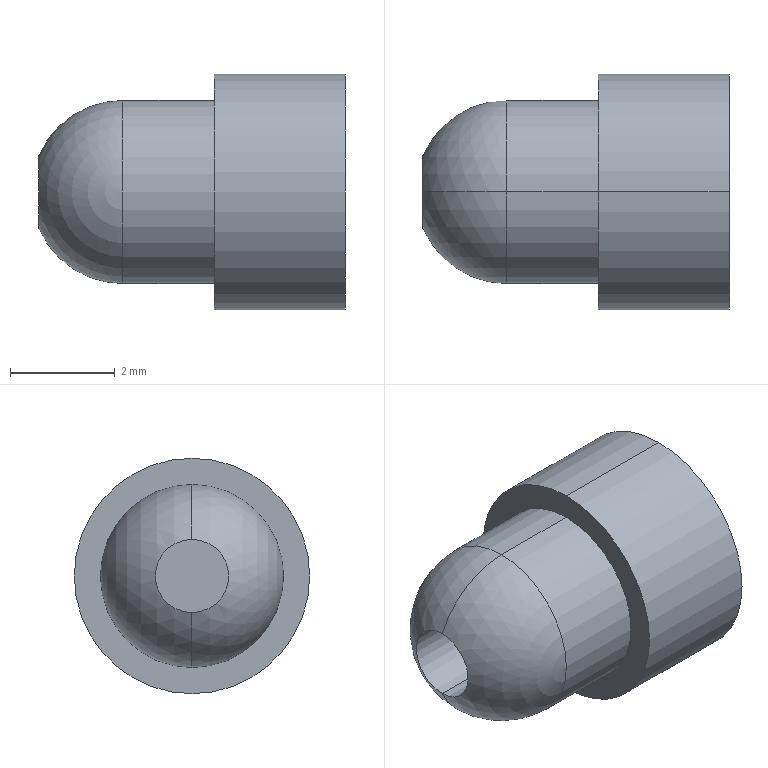Part | NX | 1 solid | 11 faces | box 5.854 x 4.5 x 4.5 mm | volume 60.236 mm3 | cylinder 6 | plane 3 | sphere 2 | commonest cylinder face diameters 1.4 x2 3.5 x2 4.5 x2
STEP:
#1=CARTESIAN_POINT('',(-7.75,0.,23.75));
#2=VERTEX_POINT('',#1);
#3=CARTESIAN_POINT('',(-7.75,0.,28.25));
#4=VERTEX_POINT('',#3);
#5=CARTESIAN_POINT('',(-7.75,0.,26.));
#6=DIRECTION('',(1.,0.,0.));
#7=DIRECTION('',(0.,0.,1.));
#8=AXIS2_PLACEMENT_3D('',#5,#6,#7);
#9=CIRCLE('',#8,2.25);
#10=EDGE_CURVE('',#2,#4,#9,.T.);
#11=ORIENTED_EDGE('',*,*,#10,.T.);
#12=CARTESIAN_POINT('',(-7.75,0.,26.));
#13=DIRECTION('',(1.,0.,0.));
#14=DIRECTION('',(0.,0.,1.));
#15=AXIS2_PLACEMENT_3D('',#12,#13,#14);
#16=CIRCLE('',#15,2.25);
#17=EDGE_CURVE('',#4,#2,#16,.T.);
#18=ORIENTED_EDGE('',*,*,#17,.T.);
#19=EDGE_LOOP('',(#11,#18));
#20=FACE_BOUND('',#19,.T.);
#21=CARTESIAN_POINT('',(-7.75,0.,26.));
#22=DIRECTION('',(1.,0.,0.));
#23=DIRECTION('',(0.,1.,0.));
#24=AXIS2_PLACEMENT_3D('',#21,#22,#23);
#25=PLANE('',#24);
#26=ADVANCED_FACE('',(#20),#25,.T.);
#27=CARTESIAN_POINT('',(-8.75,0.,25.3));
#28=VERTEX_POINT('',#27);
#29=CARTESIAN_POINT('',(-8.75,0.,26.7));
#30=VERTEX_POINT('',#29);
#31=CARTESIAN_POINT('',(-8.75,0.,26.));
#32=DIRECTION('',(-1.,0.,0.));
#33=DIRECTION('',(0.,0.,1.));
#34=AXIS2_PLACEMENT_3D('',#31,#32,#33);
#35=CIRCLE('',#34,0.7);
#36=EDGE_CURVE('',#28,#30,#35,.T.);
#37=ORIENTED_EDGE('',*,*,#36,.T.);
#38=CARTESIAN_POINT('',(-8.75,0.,26.));
#39=DIRECTION('',(-1.,0.,0.));
#40=DIRECTION('',(0.,0.,1.));
#41=AXIS2_PLACEMENT_3D('',#38,#39,#40);
#42=CIRCLE('',#41,0.7);
#43=EDGE_CURVE('',#30,#28,#42,.T.);
#44=ORIENTED_EDGE('',*,*,#43,.T.);
#45=EDGE_LOOP('',(#37,#44));
#46=FACE_BOUND('',#45,.T.);
#47=CARTESIAN_POINT('',(-8.75,0.,26.));
#48=DIRECTION('',(-1.,0.,0.));
#49=DIRECTION('',(0.,0.,1.));
#50=AXIS2_PLACEMENT_3D('',#47,#48,#49);
#51=PLANE('',#50);
#52=ADVANCED_FACE('',(#46),#51,.T.);
#53=CARTESIAN_POINT('',(-10.25,0.,28.25));
#54=VERTEX_POINT('',#53);
#55=CARTESIAN_POINT('',(-10.25,0.,23.75));
#56=VERTEX_POINT('',#55);
#57=CARTESIAN_POINT('',(-10.25,0.,26.));
#58=DIRECTION('',(-1.,0.,0.));
#59=DIRECTION('',(0.,0.,1.));
#60=AXIS2_PLACEMENT_3D('',#57,#58,#59);
#61=CIRCLE('',#60,2.25);
#62=EDGE_CURVE('',#54,#56,#61,.T.);
#63=ORIENTED_EDGE('',*,*,#62,.F.);
#64=CARTESIAN_POINT('',(-9.5,0.,28.25));
#65=DIRECTION('',(-1.,0.,0.));
#66=VECTOR('',#65,1000.);
#67=LINE('',#64,#66);
#68=EDGE_CURVE('',#4,#54,#67,.T.);
#69=ORIENTED_EDGE('',*,*,#68,.F.);
#70=ORIENTED_EDGE('',*,*,#10,.F.);
#71=CARTESIAN_POINT('',(-9.5,0.,23.75));
#72=DIRECTION('',(-1.,0.,0.));
#73=VECTOR('',#72,1000.);
#74=LINE('',#71,#73);
#75=EDGE_CURVE('',#2,#56,#74,.T.);
#76=ORIENTED_EDGE('',*,*,#75,.T.);
#77=EDGE_LOOP('',(#63,#69,#70,#76));
#78=FACE_BOUND('',#77,.T.);
#79=CARTESIAN_POINT('',(-9.5,0.,26.));
#80=DIRECTION('',(-1.,0.,0.));
#81=DIRECTION('',(0.,0.,1.));
#82=AXIS2_PLACEMENT_3D('',#79,#80,#81);
#83=CYLINDRICAL_SURFACE('',#82,2.25);
#84=ADVANCED_FACE('',(#78),#83,.T.);
#85=CARTESIAN_POINT('',(-12.,0.,24.25));
#86=VERTEX_POINT('',#85);
#87=CARTESIAN_POINT('',(-12.,0.,27.75));
#88=VERTEX_POINT('',#87);
#89=CARTESIAN_POINT('',(-12.,0.,26.));
#90=DIRECTION('',(-1.,0.,0.));
#91=DIRECTION('',(0.,0.,1.));
#92=AXIS2_PLACEMENT_3D('',#89,#90,#91);
#93=CIRCLE('',#92,1.75);
#94=EDGE_CURVE('',#86,#88,#93,.T.);
#95=ORIENTED_EDGE('',*,*,#94,.F.);
#96=CARTESIAN_POINT('',(-10.25,0.,24.25));
#97=VERTEX_POINT('',#96);
#98=CARTESIAN_POINT('',(-11.125,0.,24.25));
#99=DIRECTION('',(-1.,0.,0.));
#100=VECTOR('',#99,1000.);
#101=LINE('',#98,#100);
#102=EDGE_CURVE('',#97,#86,#101,.T.);
#103=ORIENTED_EDGE('',*,*,#102,.F.);
#104=CARTESIAN_POINT('',(-10.25,0.,27.75));
#105=VERTEX_POINT('',#104);
#106=CARTESIAN_POINT('',(-10.25,0.,26.));
#107=DIRECTION('',(-1.,0.,0.));
#108=DIRECTION('',(0.,0.,1.));
#109=AXIS2_PLACEMENT_3D('',#106,#107,#108);
#110=CIRCLE('',#109,1.75);
#111=EDGE_CURVE('',#97,#105,#110,.T.);
#112=ORIENTED_EDGE('',*,*,#111,.T.);
#113=CARTESIAN_POINT('',(-11.125,0.,27.75));
#114=DIRECTION('',(-1.,0.,0.));
#115=VECTOR('',#114,1000.);
#116=LINE('',#113,#115);
#117=EDGE_CURVE('',#105,#88,#116,.T.);
#118=ORIENTED_EDGE('',*,*,#117,.T.);
#119=EDGE_LOOP('',(#95,#103,#112,#118));
#120=FACE_BOUND('',#119,.T.);
#121=CARTESIAN_POINT('',(-11.125,0.,26.));
#122=DIRECTION('',(-1.,0.,0.));
#123=DIRECTION('',(0.,0.,1.));
#124=AXIS2_PLACEMENT_3D('',#121,#122,#123);
#125=CYLINDRICAL_SURFACE('',#124,1.75);
#126=ADVANCED_FACE('',(#120),#125,.T.);
#127=ORIENTED_EDGE('',*,*,#36,.F.);
#128=CARTESIAN_POINT('',(-13.604,0.,25.3));
#129=VERTEX_POINT('',#128);
#130=CARTESIAN_POINT('',(-11.25,0.,25.3));
#131=DIRECTION('',(-1.,0.,0.));
#132=VECTOR('',#131,1000.);
#133=LINE('',#130,#132);
#134=EDGE_CURVE('',#129,#28,#133,.F.);
#135=ORIENTED_EDGE('',*,*,#134,.F.);
#136=CARTESIAN_POINT('',(-13.604,0.,26.7));
#137=VERTEX_POINT('',#136);
#138=CARTESIAN_POINT('',(-13.604,0.,26.));
#139=DIRECTION('',(1.,0.,0.));
#140=DIRECTION('',(0.,0.,1.));
#141=AXIS2_PLACEMENT_3D('',#138,#139,#140);
#142=CIRCLE('',#141,0.7);
#143=EDGE_CURVE('',#137,#129,#142,.T.);
#144=ORIENTED_EDGE('',*,*,#143,.F.);
#145=CARTESIAN_POINT('',(-11.25,0.,26.7));
#146=DIRECTION('',(-1.,0.,0.));
#147=VECTOR('',#146,1000.);
#148=LINE('',#145,#147);
#149=EDGE_CURVE('',#137,#30,#148,.F.);
#150=ORIENTED_EDGE('',*,*,#149,.T.);
#151=EDGE_LOOP('',(#127,#135,#144,#150));
#152=FACE_BOUND('',#151,.T.);
#153=CARTESIAN_POINT('',(-11.25,0.,26.));
#154=DIRECTION('',(-1.,0.,0.));
#155=DIRECTION('',(0.,0.,1.));
#156=AXIS2_PLACEMENT_3D('',#153,#154,#155);
#157=CYLINDRICAL_SURFACE('',#156,0.7);
#158=ADVANCED_FACE('',(#152),#157,.F.);
#159=CARTESIAN_POINT('',(-12.,0.,26.));
#160=DIRECTION('',(-1.,0.,0.));
#161=DIRECTION('',(0.,0.,1.));
#162=AXIS2_PLACEMENT_3D('',#159,#160,#161);
#163=CIRCLE('',#162,1.75);
#164=EDGE_CURVE('',#88,#86,#163,.T.);
#165=ORIENTED_EDGE('',*,*,#164,.T.);
#166=CARTESIAN_POINT('',(-12.,0.,26.));
#167=DIRECTION('',(0.,1.,0.));
#168=DIRECTION('',(1.,0.,0.));
#169=AXIS2_PLACEMENT_3D('',#166,#167,#168);
#170=CIRCLE('',#169,1.75);
#171=EDGE_CURVE('',#86,#129,#170,.T.);
#172=ORIENTED_EDGE('',*,*,#171,.T.);
#173=CARTESIAN_POINT('',(-13.604,0.,26.));
#174=DIRECTION('',(1.,0.,0.));
#175=DIRECTION('',(0.,0.,1.));
#176=AXIS2_PLACEMENT_3D('',#173,#174,#175);
#177=CIRCLE('',#176,0.7);
#178=EDGE_CURVE('',#129,#137,#177,.T.);
#179=ORIENTED_EDGE('',*,*,#178,.T.);
#180=CARTESIAN_POINT('',(-12.,0.,26.));
#181=DIRECTION('',(0.,1.,0.));
#182=DIRECTION('',(1.,0.,0.));
#183=AXIS2_PLACEMENT_3D('',#180,#181,#182);
#184=CIRCLE('',#183,1.75);
#185=EDGE_CURVE('',#137,#88,#184,.T.);
#186=ORIENTED_EDGE('',*,*,#185,.T.);
#187=EDGE_LOOP('',(#165,#172,#179,#186));
#188=FACE_BOUND('',#187,.T.);
#189=CARTESIAN_POINT('',(-12.,0.,26.));
#190=DIRECTION('',(0.,1.,0.));
#191=DIRECTION('',(1.,0.,0.));
#192=AXIS2_PLACEMENT_3D('',#189,#190,#191);
#193=SPHERICAL_SURFACE('',#192,1.75);
#194=ADVANCED_FACE('',(#188),#193,.T.);
#195=ORIENTED_EDGE('',*,*,#62,.T.);
#196=CARTESIAN_POINT('',(-10.25,0.,26.));
#197=DIRECTION('',(-1.,0.,0.));
#198=DIRECTION('',(0.,0.,1.));
#199=AXIS2_PLACEMENT_3D('',#196,#197,#198);
#200=CIRCLE('',#199,2.25);
#201=EDGE_CURVE('',#56,#54,#200,.T.);
#202=ORIENTED_EDGE('',*,*,#201,.T.);
#203=EDGE_LOOP('',(#195,#202));
#204=FACE_BOUND('',#203,.T.);
#205=ORIENTED_EDGE('',*,*,#111,.F.);
#206=CARTESIAN_POINT('',(-10.25,0.,26.));
#207=DIRECTION('',(-1.,0.,0.));
#208=DIRECTION('',(0.,0.,1.));
#209=AXIS2_PLACEMENT_3D('',#206,#207,#208);
#210=CIRCLE('',#209,1.75);
#211=EDGE_CURVE('',#105,#97,#210,.T.);
#212=ORIENTED_EDGE('',*,*,#211,.F.);
#213=EDGE_LOOP('',(#205,#212));
#214=FACE_BOUND('',#213,.T.);
#215=CARTESIAN_POINT('',(-10.25,0.,28.));
#216=DIRECTION('',(-1.,0.,0.));
#217=DIRECTION('',(0.,0.,1.));
#218=AXIS2_PLACEMENT_3D('',#215,#216,#217);
#219=PLANE('',#218);
#220=ADVANCED_FACE('',(#204,#214),#219,.T.);
#221=ORIENTED_EDGE('',*,*,#68,.T.);
#222=ORIENTED_EDGE('',*,*,#201,.F.);
#223=ORIENTED_EDGE('',*,*,#75,.F.);
#224=ORIENTED_EDGE('',*,*,#17,.F.);
#225=EDGE_LOOP('',(#221,#222,#223,#224));
#226=FACE_BOUND('',#225,.T.);
#227=CARTESIAN_POINT('',(-9.5,0.,26.));
#228=DIRECTION('',(-1.,0.,0.));
#229=DIRECTION('',(0.,0.,1.));
#230=AXIS2_PLACEMENT_3D('',#227,#228,#229);
#231=CYLINDRICAL_SURFACE('',#230,2.25);
#232=ADVANCED_FACE('',(#226),#231,.T.);
#233=ORIENTED_EDGE('',*,*,#178,.F.);
#234=ORIENTED_EDGE('',*,*,#134,.T.);
#235=ORIENTED_EDGE('',*,*,#43,.F.);
#236=ORIENTED_EDGE('',*,*,#149,.F.);
#237=EDGE_LOOP('',(#233,#234,#235,#236));
#238=FACE_BOUND('',#237,.T.);
#239=CARTESIAN_POINT('',(-11.25,0.,26.));
#240=DIRECTION('',(-1.,0.,0.));
#241=DIRECTION('',(0.,0.,1.));
#242=AXIS2_PLACEMENT_3D('',#239,#240,#241);
#243=CYLINDRICAL_SURFACE('',#242,0.7);
#244=ADVANCED_FACE('',(#238),#243,.F.);
#245=ORIENTED_EDGE('',*,*,#117,.F.);
#246=ORIENTED_EDGE('',*,*,#211,.T.);
#247=ORIENTED_EDGE('',*,*,#102,.T.);
#248=ORIENTED_EDGE('',*,*,#164,.F.);
#249=EDGE_LOOP('',(#245,#246,#247,#248));
#250=FACE_BOUND('',#249,.T.);
#251=CARTESIAN_POINT('',(-11.125,0.,26.));
#252=DIRECTION('',(-1.,0.,0.));
#253=DIRECTION('',(0.,0.,1.));
#254=AXIS2_PLACEMENT_3D('',#251,#252,#253);
#255=CYLINDRICAL_SURFACE('',#254,1.75);
#256=ADVANCED_FACE('',(#250),#255,.T.);
#257=ORIENTED_EDGE('',*,*,#171,.F.);
#258=ORIENTED_EDGE('',*,*,#94,.T.);
#259=ORIENTED_EDGE('',*,*,#185,.F.);
#260=ORIENTED_EDGE('',*,*,#143,.T.);
#261=EDGE_LOOP('',(#257,#258,#259,#260));
#262=FACE_BOUND('',#261,.T.);
#263=CARTESIAN_POINT('',(-12.,0.,26.));
#264=DIRECTION('',(0.,1.,0.));
#265=DIRECTION('',(1.,0.,0.));
#266=AXIS2_PLACEMENT_3D('',#263,#264,#265);
#267=SPHERICAL_SURFACE('',#266,1.75);
#268=ADVANCED_FACE('',(#262),#267,.T.);
#269=CLOSED_SHELL('',(#26,#52,#84,#126,#158,#194,#220,#232,#244,#256,#268));
#270=MANIFOLD_SOLID_BREP('',#269);
#271=(LENGTH_UNIT()NAMED_UNIT(*)SI_UNIT(.MILLI.,.METRE.));
#272=UNCERTAINTY_MEASURE_WITH_UNIT(LENGTH_MEASURE(0.00001),#271,'','');
#273=(NAMED_UNIT(*)PLANE_ANGLE_UNIT()SI_UNIT($,.RADIAN.));
#274=(NAMED_UNIT(*)SI_UNIT($,.STERADIAN.)SOLID_ANGLE_UNIT());
#275=(GEOMETRIC_REPRESENTATION_CONTEXT(3)GLOBAL_UNCERTAINTY_ASSIGNED_CONTEXT((#272))GLOBAL_UNIT_ASSIGNED_CONTEXT((#271,#273,#274))REPRESENTATION_CONTEXT('',''));
#276=ADVANCED_BREP_SHAPE_REPRESENTATION('',(#270),#275);